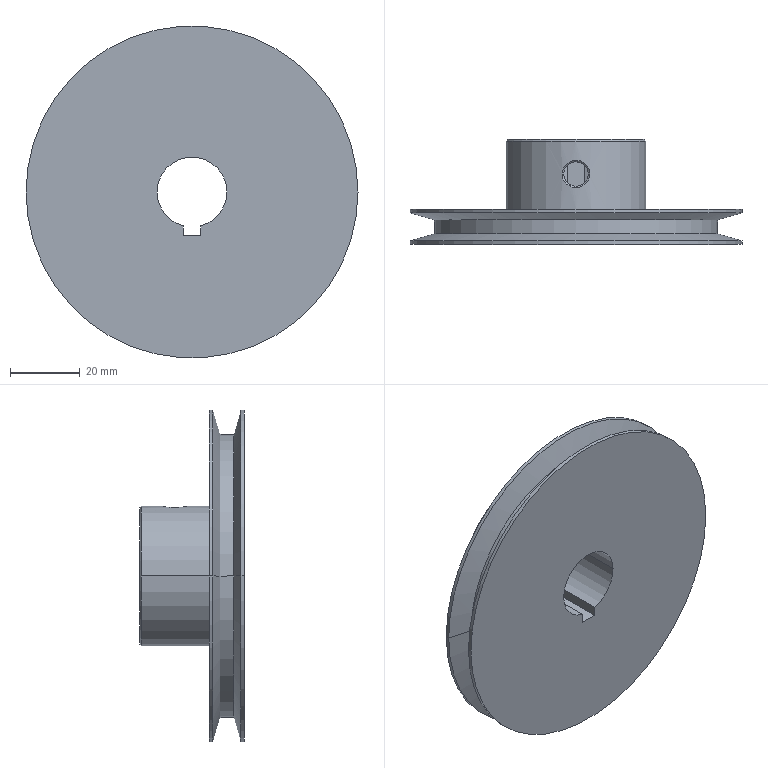Part | STEP file | BCC3 H16_3 | 1 solid | 27 faces | box 95 x 30 x 95 mm | volume 74080 mm3 | cylinder 13 | cone 6 | plane 6 | spline 2 | commonest cylinder face diameters 95 x4 20 x3 7 x2 40 x2 81 x2